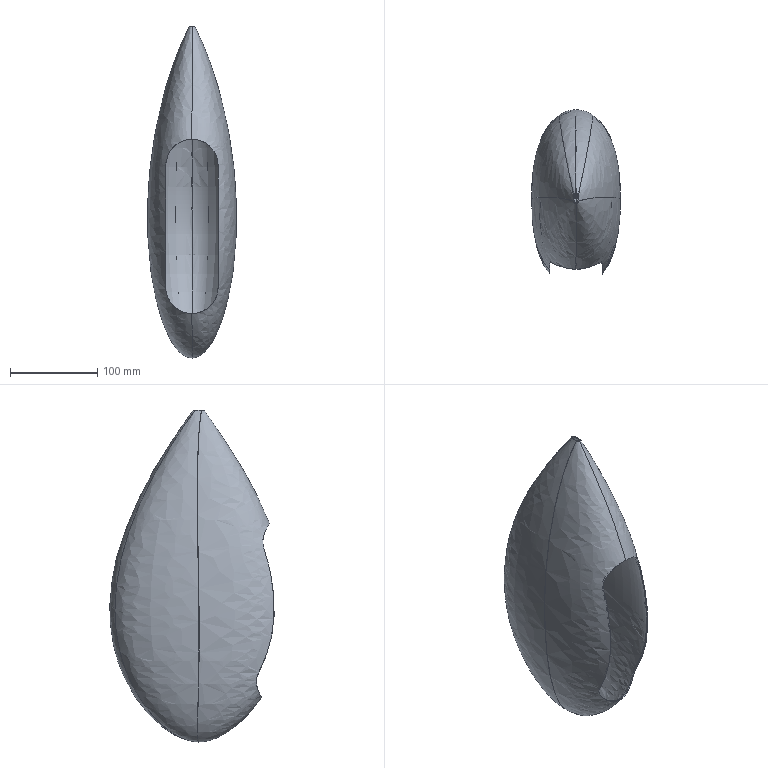Part | SolidWorks | features BaseBody 1 | 1 solid | 20 faces | volume 125666 mm3 | spline 14 | cylinder 3 | plane 3 | commonest cylinder face diameters 60 x3